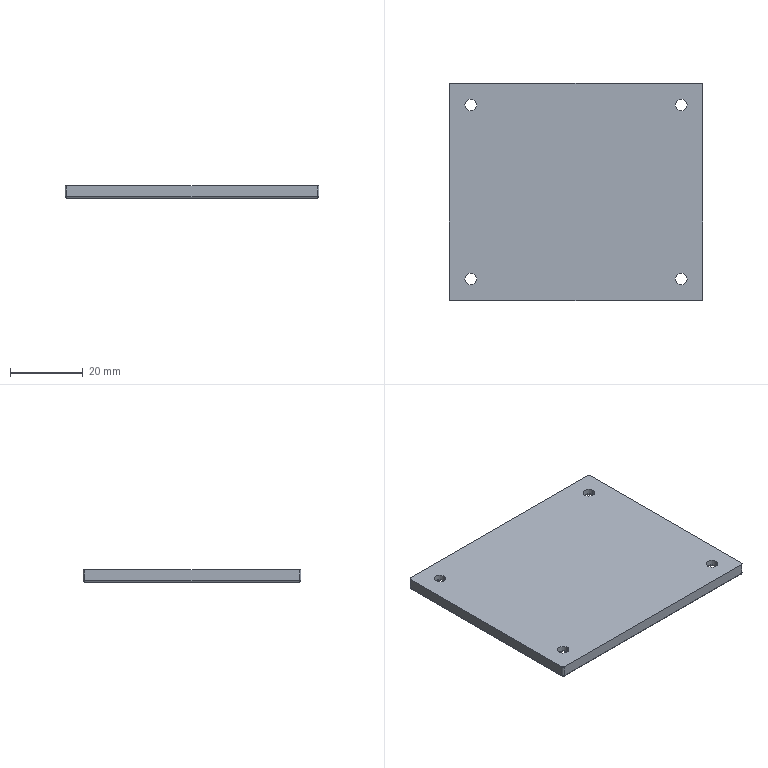Part | STEP file | Warning label | 1 solid | 4411 faces | volume 14089 mm3 | plane 2989 | spline 1382 | cylinder 36 | sphere 4 | commonest cylinder face diameters 1 x8 3.2 x8 8.5 x8 12 x6 13 x6